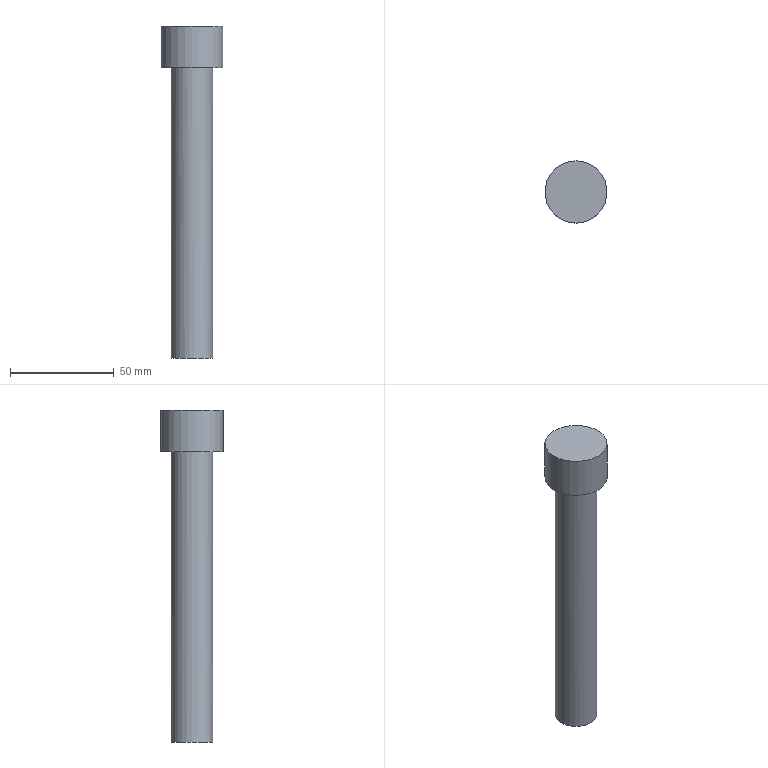Part | NX | features solid 2 | 1 solid | 5 faces | box 30 x 30 x 160 mm | volume 58119 mm3 | plane 3 | cylinder 2 | commonest cylinder face diameters 20 x1 30 x1
STEP:
#1=CARTESIAN_POINT('',(440.,590.,271.));
#2=VERTEX_POINT('',#1);
#3=CARTESIAN_POINT('',(440.,575.,271.));
#4=DIRECTION('',(0.,0.,1.));
#5=DIRECTION('',(0.,1.,0.));
#6=AXIS2_PLACEMENT_3D('',#3,#4,#5);
#7=CIRCLE('',#6,15.);
#8=EDGE_CURVE('',#2,#2,#7,.T.);
#9=ORIENTED_EDGE('',*,*,#8,.F.);
#10=EDGE_LOOP('',(#9));
#11=FACE_BOUND('',#10,.T.);
#12=CARTESIAN_POINT('',(440.,560.,251.));
#13=VERTEX_POINT('',#12);
#14=CARTESIAN_POINT('',(440.,575.,251.));
#15=DIRECTION('',(0.,0.,-1.));
#16=DIRECTION('',(0.,-1.,0.));
#17=AXIS2_PLACEMENT_3D('',#14,#15,#16);
#18=CIRCLE('',#17,15.);
#19=EDGE_CURVE('',#13,#13,#18,.F.);
#20=ORIENTED_EDGE('',*,*,#19,.T.);
#21=EDGE_LOOP('',(#20));
#22=FACE_BOUND('',#21,.T.);
#23=CARTESIAN_POINT('',(440.,575.,261.));
#24=DIRECTION('',(0.,0.,1.));
#25=DIRECTION('',(0.,-1.,0.));
#26=AXIS2_PLACEMENT_3D('',#23,#24,#25);
#27=CYLINDRICAL_SURFACE('',#26,15.);
#28=ADVANCED_FACE('',(#11,#22),#27,.T.);
#29=ORIENTED_EDGE('',*,*,#8,.T.);
#30=EDGE_LOOP('',(#29));
#31=FACE_BOUND('',#30,.T.);
#32=CARTESIAN_POINT('',(440.,575.,271.));
#33=DIRECTION('',(0.,0.,1.));
#34=DIRECTION('',(0.,-1.,0.));
#35=AXIS2_PLACEMENT_3D('',#32,#33,#34);
#36=PLANE('',#35);
#37=ADVANCED_FACE('',(#31),#36,.T.);
#38=CARTESIAN_POINT('',(440.,565.,251.));
#39=VERTEX_POINT('',#38);
#40=CARTESIAN_POINT('',(440.,575.,251.));
#41=DIRECTION('',(0.,0.,-1.));
#42=DIRECTION('',(0.,-1.,0.));
#43=AXIS2_PLACEMENT_3D('',#40,#41,#42);
#44=CIRCLE('',#43,10.);
#45=EDGE_CURVE('',#39,#39,#44,.T.);
#46=ORIENTED_EDGE('',*,*,#45,.F.);
#47=EDGE_LOOP('',(#46));
#48=FACE_BOUND('',#47,.T.);
#49=ORIENTED_EDGE('',*,*,#19,.F.);
#50=EDGE_LOOP('',(#49));
#51=FACE_BOUND('',#50,.T.);
#52=CARTESIAN_POINT('',(440.,575.,251.));
#53=DIRECTION('',(0.,0.,1.));
#54=DIRECTION('',(0.,-1.,0.));
#55=AXIS2_PLACEMENT_3D('',#52,#53,#54);
#56=PLANE('',#55);
#57=ADVANCED_FACE('',(#48,#51),#56,.F.);
#58=CARTESIAN_POINT('',(430.,575.,111.));
#59=VERTEX_POINT('',#58);
#60=CARTESIAN_POINT('',(440.,575.,111.));
#61=DIRECTION('',(0.,0.,-1.));
#62=DIRECTION('',(-1.,0.,0.));
#63=AXIS2_PLACEMENT_3D('',#60,#61,#62);
#64=CIRCLE('',#63,10.);
#65=EDGE_CURVE('',#59,#59,#64,.T.);
#66=ORIENTED_EDGE('',*,*,#65,.T.);
#67=EDGE_LOOP('',(#66));
#68=FACE_BOUND('',#67,.T.);
#69=CARTESIAN_POINT('',(440.,575.,111.));
#70=DIRECTION('',(0.,0.,-1.));
#71=DIRECTION('',(0.,1.,0.));
#72=AXIS2_PLACEMENT_3D('',#69,#70,#71);
#73=PLANE('',#72);
#74=ADVANCED_FACE('',(#68),#73,.T.);
#75=ORIENTED_EDGE('',*,*,#65,.F.);
#76=EDGE_LOOP('',(#75));
#77=FACE_BOUND('',#76,.T.);
#78=ORIENTED_EDGE('',*,*,#45,.T.);
#79=EDGE_LOOP('',(#78));
#80=FACE_BOUND('',#79,.T.);
#81=CARTESIAN_POINT('',(440.,575.,145.));
#82=DIRECTION('',(0.,0.,-1.));
#83=DIRECTION('',(0.,1.,0.));
#84=AXIS2_PLACEMENT_3D('',#81,#82,#83);
#85=CYLINDRICAL_SURFACE('',#84,10.);
#86=ADVANCED_FACE('',(#77,#80),#85,.T.);
#87=CLOSED_SHELL('',(#28,#37,#57,#74,#86));
#88=MANIFOLD_SOLID_BREP('',#87);
#89=(LENGTH_UNIT()NAMED_UNIT(*)SI_UNIT(.MILLI.,.METRE.));
#90=UNCERTAINTY_MEASURE_WITH_UNIT(LENGTH_MEASURE(0.00001),#89,'','');
#91=(NAMED_UNIT(*)PLANE_ANGLE_UNIT()SI_UNIT($,.RADIAN.));
#92=(NAMED_UNIT(*)SI_UNIT($,.STERADIAN.)SOLID_ANGLE_UNIT());
#93=(GEOMETRIC_REPRESENTATION_CONTEXT(3)GLOBAL_UNCERTAINTY_ASSIGNED_CONTEXT((#90))GLOBAL_UNIT_ASSIGNED_CONTEXT((#89,#91,#92))REPRESENTATION_CONTEXT('',''));
#94=ADVANCED_BREP_SHAPE_REPRESENTATION('',(#88),#93);